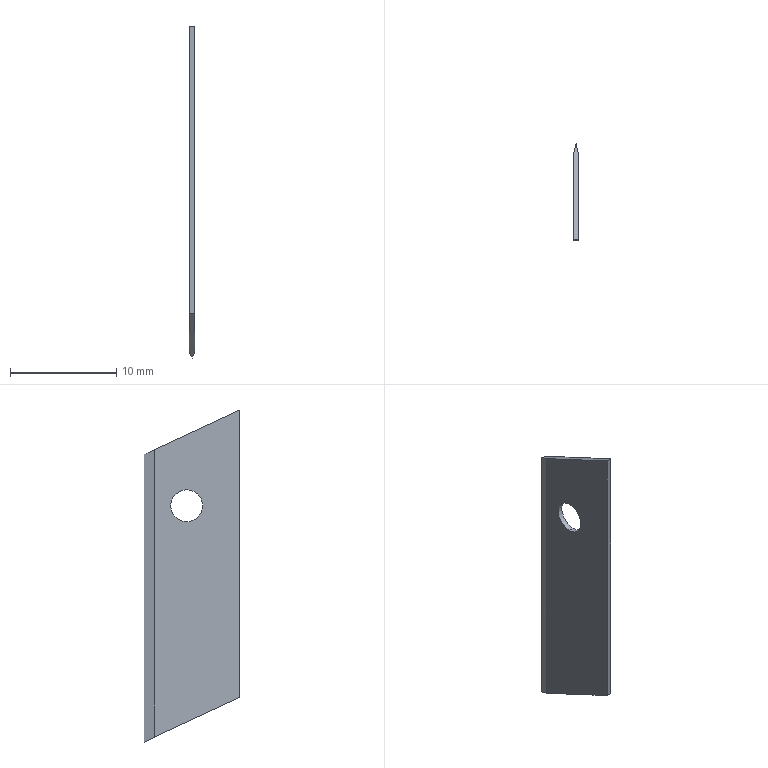Part | STEP file | Insert blade | 1 solid | 9 faces | box 0.5 x 9 x 31.197 mm | volume 111.216 mm3 | plane 7 | cylinder 2 | commonest cylinder face diameters 3 x2
STEP:
#1=CARTESIAN_POINT('',(0.,0.,0.));
#2=DIRECTION('',(0.,0.,1.));
#3=DIRECTION('',(1.,0.,0.));
#4=AXIS2_PLACEMENT_3D('',#1,#2,#3);
#5=CARTESIAN_POINT('',(-0.25,5.,-10.5));
#6=VERTEX_POINT('',#5);
#7=CARTESIAN_POINT('',(0.25,5.,-10.5));
#8=VERTEX_POINT('',#7);
#9=CARTESIAN_POINT('',(-0.25,5.,-10.5));
#10=DIRECTION('',(1.,0.,0.));
#11=VECTOR('',#10,1.);
#12=LINE('',#9,#11);
#13=CARTESIAN_POINT('',(-0.25,5.,-9.));
#14=DIRECTION('',(1.,0.,0.));
#15=DIRECTION('',(0.,0.,-1.));
#16=AXIS2_PLACEMENT_3D('',#13,#14,#15);
#17=CYLINDRICAL_SURFACE('',#16,1.5);
#18=CARTESIAN_POINT('',(6.283,0.));
#19=DIRECTION('',(0.,1.));
#20=VECTOR('',#19,1.);
#21=LINE('',#18,#20);
#22=(GEOMETRIC_REPRESENTATION_CONTEXT(2)PARAMETRIC_REPRESENTATION_CONTEXT()REPRESENTATION_CONTEXT('',''));
#23=DEFINITIONAL_REPRESENTATION('',(#21),#22);
#24=PCURVE('',#17,#23);
#25=CARTESIAN_POINT('',(-0.25,5.,-9.));
#26=DIRECTION('',(1.,0.,0.));
#27=DIRECTION('',(0.,0.,-1.));
#28=AXIS2_PLACEMENT_3D('',#25,#26,#27);
#29=CYLINDRICAL_SURFACE('',#28,1.5);
#30=CARTESIAN_POINT('',(0.,0.));
#31=DIRECTION('',(0.,1.));
#32=VECTOR('',#31,1.);
#33=LINE('',#30,#32);
#34=(GEOMETRIC_REPRESENTATION_CONTEXT(2)PARAMETRIC_REPRESENTATION_CONTEXT()REPRESENTATION_CONTEXT('',''));
#35=DEFINITIONAL_REPRESENTATION('',(#33),#34);
#36=PCURVE('',#29,#35);
#37=SURFACE_CURVE('',#12,(#24,#36),.PCURVE_S1.);
#38=EDGE_CURVE('',#6,#8,#37,.T.);
#39=ORIENTED_EDGE('',*,*,#38,.T.);
#40=CARTESIAN_POINT('',(0.25,5.,-7.5));
#41=VERTEX_POINT('',#40);
#42=CARTESIAN_POINT('',(0.25,5.,-9.));
#43=DIRECTION('',(1.,0.,0.));
#44=DIRECTION('',(0.,0.,-1.));
#45=AXIS2_PLACEMENT_3D('',#42,#43,#44);
#46=CIRCLE('',#45,1.5);
#47=CARTESIAN_POINT('',(0.,0.5));
#48=DIRECTION('',(1.,0.));
#49=VECTOR('',#48,1.);
#50=LINE('',#47,#49);
#51=(GEOMETRIC_REPRESENTATION_CONTEXT(2)PARAMETRIC_REPRESENTATION_CONTEXT()REPRESENTATION_CONTEXT('',''));
#52=DEFINITIONAL_REPRESENTATION('',(#50),#51);
#53=PCURVE('',#17,#52);
#54=CARTESIAN_POINT('',(0.25,0.,-30.915));
#55=DIRECTION('',(-1.,0.,0.));
#56=DIRECTION('',(0.,0.,1.));
#57=AXIS2_PLACEMENT_3D('',#54,#55,#56);
#58=PLANE('',#57);
#59=CARTESIAN_POINT('',(20.415,5.));
#60=CARTESIAN_POINT('',(20.415,7.598));
#61=CARTESIAN_POINT('',(22.665,6.299));
#62=CARTESIAN_POINT('',(24.915,5.));
#63=CARTESIAN_POINT('',(22.665,3.701));
#64=CARTESIAN_POINT('',(20.415,2.402));
#65=CARTESIAN_POINT('',(20.415,5.));
#66=(BOUNDED_CURVE()B_SPLINE_CURVE(2,(#59,#60,#61,#62,#63,#64,#65),.UNSPECIFIED.,.T.,.F.)B_SPLINE_CURVE_WITH_KNOTS((1,2,2,2,2,1),(-2.094,0.,2.094,4.189,6.283,8.378),.UNSPECIFIED.)CURVE()GEOMETRIC_REPRESENTATION_ITEM()RATIONAL_B_SPLINE_CURVE((1.,0.5,1.,0.5,1.,0.5,1.))REPRESENTATION_ITEM(''));
#67=(GEOMETRIC_REPRESENTATION_CONTEXT(2)PARAMETRIC_REPRESENTATION_CONTEXT()REPRESENTATION_CONTEXT('',''));
#68=DEFINITIONAL_REPRESENTATION('',(#66),#67);
#69=PCURVE('',#58,#68);
#70=SURFACE_CURVE('',#46,(#53,#69),.PCURVE_S1.);
#71=EDGE_CURVE('',#41,#8,#70,.T.);
#72=ORIENTED_EDGE('',*,*,#71,.F.);
#73=CARTESIAN_POINT('',(-0.25,5.,-7.5));
#74=VERTEX_POINT('',#73);
#75=CARTESIAN_POINT('',(-0.25,5.,-7.5));
#76=DIRECTION('',(1.,0.,0.));
#77=VECTOR('',#76,1.);
#78=LINE('',#75,#77);
#79=CARTESIAN_POINT('',(3.142,0.));
#80=DIRECTION('',(0.,1.));
#81=VECTOR('',#80,1.);
#82=LINE('',#79,#81);
#83=(GEOMETRIC_REPRESENTATION_CONTEXT(2)PARAMETRIC_REPRESENTATION_CONTEXT()REPRESENTATION_CONTEXT('',''));
#84=DEFINITIONAL_REPRESENTATION('',(#82),#83);
#85=PCURVE('',#17,#84);
#86=CARTESIAN_POINT('',(3.142,0.));
#87=DIRECTION('',(0.,1.));
#88=VECTOR('',#87,1.);
#89=LINE('',#86,#88);
#90=(GEOMETRIC_REPRESENTATION_CONTEXT(2)PARAMETRIC_REPRESENTATION_CONTEXT()REPRESENTATION_CONTEXT('',''));
#91=DEFINITIONAL_REPRESENTATION('',(#89),#90);
#92=PCURVE('',#29,#91);
#93=SURFACE_CURVE('',#78,(#85,#92),.PCURVE_S1.);
#94=EDGE_CURVE('',#74,#41,#93,.T.);
#95=ORIENTED_EDGE('',*,*,#94,.F.);
#96=CARTESIAN_POINT('',(-0.25,5.,-9.));
#97=DIRECTION('',(-1.,0.,0.));
#98=DIRECTION('',(0.,0.,-1.));
#99=AXIS2_PLACEMENT_3D('',#96,#97,#98);
#100=CIRCLE('',#99,1.5);
#101=CARTESIAN_POINT('',(6.283,0.));
#102=DIRECTION('',(-1.,0.));
#103=VECTOR('',#102,1.);
#104=LINE('',#101,#103);
#105=(GEOMETRIC_REPRESENTATION_CONTEXT(2)PARAMETRIC_REPRESENTATION_CONTEXT()REPRESENTATION_CONTEXT('',''));
#106=DEFINITIONAL_REPRESENTATION('',(#104),#105);
#107=PCURVE('',#17,#106);
#108=CARTESIAN_POINT('',(-0.25,0.,-30.915));
#109=DIRECTION('',(-1.,0.,0.));
#110=DIRECTION('',(0.,0.,1.));
#111=AXIS2_PLACEMENT_3D('',#108,#109,#110);
#112=PLANE('',#111);
#113=CARTESIAN_POINT('',(21.915,5.));
#114=DIRECTION('',(-1.,0.));
#115=AXIS2_PLACEMENT_2D('',#113,#114);
#116=CIRCLE('',#115,1.5);
#117=(GEOMETRIC_REPRESENTATION_CONTEXT(2)PARAMETRIC_REPRESENTATION_CONTEXT()REPRESENTATION_CONTEXT('',''));
#118=DEFINITIONAL_REPRESENTATION('',(#116),#117);
#119=PCURVE('',#112,#118);
#120=SURFACE_CURVE('',#100,(#107,#119),.PCURVE_S1.);
#121=EDGE_CURVE('',#6,#74,#120,.T.);
#122=ORIENTED_EDGE('',*,*,#121,.F.);
#123=EDGE_LOOP('',(#39,#72,#95,#122));
#124=FACE_BOUND('',#123,.F.);
#125=ADVANCED_FACE('',(#124),#17,.F.);
#126=CARTESIAN_POINT('',(0.25,5.,-9.));
#127=DIRECTION('',(1.,0.,0.));
#128=DIRECTION('',(0.,0.,-1.));
#129=AXIS2_PLACEMENT_3D('',#126,#127,#128);
#130=CIRCLE('',#129,1.5);
#131=CARTESIAN_POINT('',(0.,0.5));
#132=DIRECTION('',(1.,0.));
#133=VECTOR('',#132,1.);
#134=LINE('',#131,#133);
#135=(GEOMETRIC_REPRESENTATION_CONTEXT(2)PARAMETRIC_REPRESENTATION_CONTEXT()REPRESENTATION_CONTEXT('',''));
#136=DEFINITIONAL_REPRESENTATION('',(#134),#135);
#137=PCURVE('',#29,#136);
#138=CARTESIAN_POINT('',(20.415,5.));
#139=CARTESIAN_POINT('',(20.415,7.598));
#140=CARTESIAN_POINT('',(22.665,6.299));
#141=CARTESIAN_POINT('',(24.915,5.));
#142=CARTESIAN_POINT('',(22.665,3.701));
#143=CARTESIAN_POINT('',(20.415,2.402));
#144=CARTESIAN_POINT('',(20.415,5.));
#145=(BOUNDED_CURVE()B_SPLINE_CURVE(2,(#138,#139,#140,#141,#142,#143,#144),.UNSPECIFIED.,.T.,.F.)B_SPLINE_CURVE_WITH_KNOTS((1,2,2,2,2,1),(-2.094,0.,2.094,4.189,6.283,8.378),.UNSPECIFIED.)CURVE()GEOMETRIC_REPRESENTATION_ITEM()RATIONAL_B_SPLINE_CURVE((1.,0.5,1.,0.5,1.,0.5,1.))REPRESENTATION_ITEM(''));
#146=(GEOMETRIC_REPRESENTATION_CONTEXT(2)PARAMETRIC_REPRESENTATION_CONTEXT()REPRESENTATION_CONTEXT('',''));
#147=DEFINITIONAL_REPRESENTATION('',(#145),#146);
#148=PCURVE('',#58,#147);
#149=SURFACE_CURVE('',#130,(#137,#148),.PCURVE_S1.);
#150=EDGE_CURVE('',#8,#41,#149,.T.);
#151=ORIENTED_EDGE('',*,*,#150,.F.);
#152=ORIENTED_EDGE('',*,*,#38,.F.);
#153=CARTESIAN_POINT('',(-0.25,5.,-9.));
#154=DIRECTION('',(-1.,0.,0.));
#155=DIRECTION('',(0.,0.,-1.));
#156=AXIS2_PLACEMENT_3D('',#153,#154,#155);
#157=CIRCLE('',#156,1.5);
#158=CARTESIAN_POINT('',(6.283,0.));
#159=DIRECTION('',(-1.,0.));
#160=VECTOR('',#159,1.);
#161=LINE('',#158,#160);
#162=(GEOMETRIC_REPRESENTATION_CONTEXT(2)PARAMETRIC_REPRESENTATION_CONTEXT()REPRESENTATION_CONTEXT('',''));
#163=DEFINITIONAL_REPRESENTATION('',(#161),#162);
#164=PCURVE('',#29,#163);
#165=CARTESIAN_POINT('',(21.915,5.));
#166=DIRECTION('',(-1.,0.));
#167=AXIS2_PLACEMENT_2D('',#165,#166);
#168=CIRCLE('',#167,1.5);
#169=(GEOMETRIC_REPRESENTATION_CONTEXT(2)PARAMETRIC_REPRESENTATION_CONTEXT()REPRESENTATION_CONTEXT('',''));
#170=DEFINITIONAL_REPRESENTATION('',(#168),#169);
#171=PCURVE('',#112,#170);
#172=SURFACE_CURVE('',#157,(#164,#171),.PCURVE_S1.);
#173=EDGE_CURVE('',#74,#6,#172,.T.);
#174=ORIENTED_EDGE('',*,*,#173,.F.);
#175=ORIENTED_EDGE('',*,*,#94,.T.);
#176=EDGE_LOOP('',(#151,#152,#174,#175));
#177=FACE_BOUND('',#176,.F.);
#178=ADVANCED_FACE('',(#177),#29,.F.);
#179=ORIENTED_EDGE('',*,*,#150,.F.);
#180=ORIENTED_EDGE('',*,*,#71,.F.);
#181=EDGE_LOOP('',(#179,#180));
#182=FACE_BOUND('',#181,.T.);
#183=CARTESIAN_POINT('',(0.25,8.,-3.73));
#184=VERTEX_POINT('',#183);
#185=CARTESIAN_POINT('',(0.25,8.,-30.73));
#186=VERTEX_POINT('',#185);
#187=CARTESIAN_POINT('',(0.25,8.,-15.365));
#188=DIRECTION('',(0.,0.,-1.));
#189=VECTOR('',#188,1.);
#190=LINE('',#187,#189);
#191=CARTESIAN_POINT('',(15.55,8.));
#192=DIRECTION('',(-1.,0.));
#193=VECTOR('',#192,1.);
#194=LINE('',#191,#193);
#195=(GEOMETRIC_REPRESENTATION_CONTEXT(2)PARAMETRIC_REPRESENTATION_CONTEXT()REPRESENTATION_CONTEXT('',''));
#196=DEFINITIONAL_REPRESENTATION('',(#194),#195);
#197=PCURVE('',#58,#196);
#198=CARTESIAN_POINT('',(0.,9.,-31.362));
#199=DIRECTION('',(-0.9701,-0.2425,0.));
#200=DIRECTION('',(0.2425,-0.9701,0.));
#201=AXIS2_PLACEMENT_3D('',#198,#199,#200);
#202=PLANE('',#201);
#203=CARTESIAN_POINT('',(1.031,15.996));
#204=DIRECTION('',(0.,-1.));
#205=VECTOR('',#204,1.);
#206=LINE('',#203,#205);
#207=(GEOMETRIC_REPRESENTATION_CONTEXT(2)PARAMETRIC_REPRESENTATION_CONTEXT()REPRESENTATION_CONTEXT('',''));
#208=DEFINITIONAL_REPRESENTATION('',(#206),#207);
#209=PCURVE('',#202,#208);
#210=SURFACE_CURVE('',#190,(#197,#209),.PCURVE_S1.);
#211=EDGE_CURVE('',#184,#186,#210,.T.);
#212=ORIENTED_EDGE('',*,*,#211,.F.);
#213=CARTESIAN_POINT('',(0.25,0.,0.));
#214=VERTEX_POINT('',#213);
#215=CARTESIAN_POINT('',(0.25,0.,0.));
#216=DIRECTION('',(0.,0.9063,-0.4226));
#217=VECTOR('',#216,1.);
#218=LINE('',#215,#217);
#219=CARTESIAN_POINT('',(30.915,0.));
#220=DIRECTION('',(-0.4226,0.9063));
#221=VECTOR('',#220,1.);
#222=LINE('',#219,#221);
#223=(GEOMETRIC_REPRESENTATION_CONTEXT(2)PARAMETRIC_REPRESENTATION_CONTEXT()REPRESENTATION_CONTEXT('',''));
#224=DEFINITIONAL_REPRESENTATION('',(#222),#223);
#225=PCURVE('',#58,#224);
#226=CARTESIAN_POINT('',(-0.25,0.,0.));
#227=DIRECTION('',(0.,-0.4226,-0.9063));
#228=DIRECTION('',(0.,0.9063,-0.4226));
#229=AXIS2_PLACEMENT_3D('',#226,#227,#228);
#230=PLANE('',#229);
#231=CARTESIAN_POINT('',(0.,0.5));
#232=DIRECTION('',(1.,0.));
#233=VECTOR('',#232,1.);
#234=LINE('',#231,#233);
#235=(GEOMETRIC_REPRESENTATION_CONTEXT(2)PARAMETRIC_REPRESENTATION_CONTEXT()REPRESENTATION_CONTEXT('',''));
#236=DEFINITIONAL_REPRESENTATION('',(#234),#235);
#237=PCURVE('',#230,#236);
#238=SURFACE_CURVE('',#218,(#225,#237),.PCURVE_S1.);
#239=EDGE_CURVE('',#214,#184,#238,.T.);
#240=ORIENTED_EDGE('',*,*,#239,.F.);
#241=CARTESIAN_POINT('',(0.25,0.,-27.));
#242=VERTEX_POINT('',#241);
#243=CARTESIAN_POINT('',(0.25,0.,-15.365));
#244=DIRECTION('',(0.,0.,1.));
#245=VECTOR('',#244,1.);
#246=LINE('',#243,#245);
#247=CARTESIAN_POINT('',(15.55,0.));
#248=DIRECTION('',(1.,0.));
#249=VECTOR('',#248,1.);
#250=LINE('',#247,#249);
#251=(GEOMETRIC_REPRESENTATION_CONTEXT(2)PARAMETRIC_REPRESENTATION_CONTEXT()REPRESENTATION_CONTEXT('',''));
#252=DEFINITIONAL_REPRESENTATION('',(#250),#251);
#253=PCURVE('',#58,#252);
#254=CARTESIAN_POINT('',(-0.25,0.,-27.));
#255=DIRECTION('',(0.,1.,0.));
#256=DIRECTION('',(0.,0.,1.));
#257=AXIS2_PLACEMENT_3D('',#254,#255,#256);
#258=PLANE('',#257);
#259=CARTESIAN_POINT('',(11.635,0.5));
#260=DIRECTION('',(1.,0.));
#261=VECTOR('',#260,1.);
#262=LINE('',#259,#261);
#263=(GEOMETRIC_REPRESENTATION_CONTEXT(2)PARAMETRIC_REPRESENTATION_CONTEXT()REPRESENTATION_CONTEXT('',''));
#264=DEFINITIONAL_REPRESENTATION('',(#262),#263);
#265=PCURVE('',#258,#264);
#266=SURFACE_CURVE('',#246,(#253,#265),.PCURVE_S1.);
#267=EDGE_CURVE('',#242,#214,#266,.T.);
#268=ORIENTED_EDGE('',*,*,#267,.F.);
#269=CARTESIAN_POINT('',(0.25,9.,-31.197));
#270=DIRECTION('',(0.,-0.9063,0.4226));
#271=VECTOR('',#270,1.);
#272=LINE('',#269,#271);
#273=CARTESIAN_POINT('',(-0.2819,9.));
#274=DIRECTION('',(0.4226,-0.9063));
#275=VECTOR('',#274,1.);
#276=LINE('',#273,#275);
#277=(GEOMETRIC_REPRESENTATION_CONTEXT(2)PARAMETRIC_REPRESENTATION_CONTEXT()REPRESENTATION_CONTEXT('',''));
#278=DEFINITIONAL_REPRESENTATION('',(#276),#277);
#279=PCURVE('',#58,#278);
#280=CARTESIAN_POINT('',(-0.25,9.,-31.197));
#281=DIRECTION('',(0.,0.4226,0.9063));
#282=DIRECTION('',(0.,-0.9063,0.4226));
#283=AXIS2_PLACEMENT_3D('',#280,#281,#282);
#284=PLANE('',#283);
#285=CARTESIAN_POINT('',(0.,0.5));
#286=DIRECTION('',(1.,0.));
#287=VECTOR('',#286,1.);
#288=LINE('',#285,#287);
#289=(GEOMETRIC_REPRESENTATION_CONTEXT(2)PARAMETRIC_REPRESENTATION_CONTEXT()REPRESENTATION_CONTEXT('',''));
#290=DEFINITIONAL_REPRESENTATION('',(#288),#289);
#291=PCURVE('',#284,#290);
#292=SURFACE_CURVE('',#272,(#279,#291),.PCURVE_S1.);
#293=EDGE_CURVE('',#186,#242,#292,.T.);
#294=ORIENTED_EDGE('',*,*,#293,.F.);
#295=EDGE_LOOP('',(#212,#240,#268,#294));
#296=FACE_BOUND('',#295,.T.);
#297=ADVANCED_FACE('',(#182,#296),#58,.F.);
#298=ORIENTED_EDGE('',*,*,#121,.F.);
#299=ORIENTED_EDGE('',*,*,#173,.F.);
#300=EDGE_LOOP('',(#298,#299));
#301=FACE_BOUND('',#300,.T.);
#302=CARTESIAN_POINT('',(-0.25,8.,-30.73));
#303=VERTEX_POINT('',#302);
#304=CARTESIAN_POINT('',(-0.25,0.,-27.));
#305=VERTEX_POINT('',#304);
#306=CARTESIAN_POINT('',(-0.25,8.,-30.73));
#307=DIRECTION('',(0.,-0.9063,0.4226));
#308=VECTOR('',#307,1.);
#309=LINE('',#306,#308);
#310=CARTESIAN_POINT('',(0.1844,8.));
#311=DIRECTION('',(0.4226,-0.9063));
#312=VECTOR('',#311,1.);
#313=LINE('',#310,#312);
#314=(GEOMETRIC_REPRESENTATION_CONTEXT(2)PARAMETRIC_REPRESENTATION_CONTEXT()REPRESENTATION_CONTEXT('',''));
#315=DEFINITIONAL_REPRESENTATION('',(#313),#314);
#316=PCURVE('',#112,#315);
#317=CARTESIAN_POINT('',(1.103,0.));
#318=DIRECTION('',(1.,0.));
#319=VECTOR('',#318,1.);
#320=LINE('',#317,#319);
#321=(GEOMETRIC_REPRESENTATION_CONTEXT(2)PARAMETRIC_REPRESENTATION_CONTEXT()REPRESENTATION_CONTEXT('',''));
#322=DEFINITIONAL_REPRESENTATION('',(#320),#321);
#323=PCURVE('',#284,#322);
#324=SURFACE_CURVE('',#309,(#316,#323),.PCURVE_S1.);
#325=EDGE_CURVE('',#303,#305,#324,.T.);
#326=ORIENTED_EDGE('',*,*,#325,.T.);
#327=CARTESIAN_POINT('',(-0.25,0.,-0.000000004));
#328=VERTEX_POINT('',#327);
#329=CARTESIAN_POINT('',(-0.25,0.,-15.365));
#330=DIRECTION('',(0.,0.,1.));
#331=VECTOR('',#330,1.);
#332=LINE('',#329,#331);
#333=CARTESIAN_POINT('',(15.55,0.));
#334=DIRECTION('',(1.,0.));
#335=VECTOR('',#334,1.);
#336=LINE('',#333,#335);
#337=(GEOMETRIC_REPRESENTATION_CONTEXT(2)PARAMETRIC_REPRESENTATION_CONTEXT()REPRESENTATION_CONTEXT('',''));
#338=DEFINITIONAL_REPRESENTATION('',(#336),#337);
#339=PCURVE('',#112,#338);
#340=CARTESIAN_POINT('',(11.635,0.));
#341=DIRECTION('',(1.,0.));
#342=VECTOR('',#341,1.);
#343=LINE('',#340,#342);
#344=(GEOMETRIC_REPRESENTATION_CONTEXT(2)PARAMETRIC_REPRESENTATION_CONTEXT()REPRESENTATION_CONTEXT('',''));
#345=DEFINITIONAL_REPRESENTATION('',(#343),#344);
#346=PCURVE('',#258,#345);
#347=SURFACE_CURVE('',#332,(#339,#346),.PCURVE_S1.);
#348=EDGE_CURVE('',#305,#328,#347,.T.);
#349=ORIENTED_EDGE('',*,*,#348,.T.);
#350=CARTESIAN_POINT('',(-0.25,8.,-3.73));
#351=VERTEX_POINT('',#350);
#352=CARTESIAN_POINT('',(-0.25,0.,-0.000000007));
#353=DIRECTION('',(0.,0.9063,-0.4226));
#354=VECTOR('',#353,1.);
#355=LINE('',#352,#354);
#356=CARTESIAN_POINT('',(30.915,0.));
#357=DIRECTION('',(-0.4226,0.9063));
#358=VECTOR('',#357,1.);
#359=LINE('',#356,#358);
#360=(GEOMETRIC_REPRESENTATION_CONTEXT(2)PARAMETRIC_REPRESENTATION_CONTEXT()REPRESENTATION_CONTEXT('',''));
#361=DEFINITIONAL_REPRESENTATION('',(#359),#360);
#362=PCURVE('',#112,#361);
#363=CARTESIAN_POINT('',(0.000000003,0.));
#364=DIRECTION('',(1.,0.));
#365=VECTOR('',#364,1.);
#366=LINE('',#363,#365);
#367=(GEOMETRIC_REPRESENTATION_CONTEXT(2)PARAMETRIC_REPRESENTATION_CONTEXT()REPRESENTATION_CONTEXT('',''));
#368=DEFINITIONAL_REPRESENTATION('',(#366),#367);
#369=PCURVE('',#230,#368);
#370=SURFACE_CURVE('',#355,(#362,#369),.PCURVE_S1.);
#371=EDGE_CURVE('',#328,#351,#370,.T.);
#372=ORIENTED_EDGE('',*,*,#371,.T.);
#373=CARTESIAN_POINT('',(-0.25,8.,-15.365));
#374=DIRECTION('',(0.,0.,-1.));
#375=VECTOR('',#374,1.);
#376=LINE('',#373,#375);
#377=CARTESIAN_POINT('',(15.55,8.));
#378=DIRECTION('',(-1.,0.));
#379=VECTOR('',#378,1.);
#380=LINE('',#377,#379);
#381=(GEOMETRIC_REPRESENTATION_CONTEXT(2)PARAMETRIC_REPRESENTATION_CONTEXT()REPRESENTATION_CONTEXT('',''));
#382=DEFINITIONAL_REPRESENTATION('',(#380),#381);
#383=PCURVE('',#112,#382);
#384=CARTESIAN_POINT('',(0.,9.,-31.362));
#385=DIRECTION('',(-0.9701,0.2425,0.));
#386=DIRECTION('',(-0.2425,-0.9701,0.));
#387=AXIS2_PLACEMENT_3D('',#384,#385,#386);
#388=PLANE('',#387);
#389=CARTESIAN_POINT('',(1.031,15.996));
#390=DIRECTION('',(0.,-1.));
#391=VECTOR('',#390,1.);
#392=LINE('',#389,#391);
#393=(GEOMETRIC_REPRESENTATION_CONTEXT(2)PARAMETRIC_REPRESENTATION_CONTEXT()REPRESENTATION_CONTEXT('',''));
#394=DEFINITIONAL_REPRESENTATION('',(#392),#393);
#395=PCURVE('',#388,#394);
#396=SURFACE_CURVE('',#376,(#383,#395),.PCURVE_S1.);
#397=EDGE_CURVE('',#351,#303,#396,.T.);
#398=ORIENTED_EDGE('',*,*,#397,.T.);
#399=EDGE_LOOP('',(#326,#349,#372,#398));
#400=FACE_BOUND('',#399,.T.);
#401=ADVANCED_FACE('',(#301,#400),#112,.T.);
#402=CARTESIAN_POINT('',(0.,9.,-31.197));
#403=VERTEX_POINT('',#402);
#404=CARTESIAN_POINT('',(0.,9.,-31.197));
#405=DIRECTION('',(-0.221,-0.8839,0.4122));
#406=VECTOR('',#405,1.);
#407=LINE('',#404,#406);
#408=CARTESIAN_POINT('',(0.,0.25));
#409=DIRECTION('',(0.9753,-0.221));
#410=VECTOR('',#409,1.);
#411=LINE('',#408,#410);
#412=(GEOMETRIC_REPRESENTATION_CONTEXT(2)PARAMETRIC_REPRESENTATION_CONTEXT()REPRESENTATION_CONTEXT('',''));
#413=DEFINITIONAL_REPRESENTATION('',(#411),#412);
#414=PCURVE('',#284,#413);
#415=CARTESIAN_POINT('',(0.,0.1648));
#416=DIRECTION('',(0.9111,0.4122));
#417=VECTOR('',#416,1.);
#418=LINE('',#415,#417);
#419=(GEOMETRIC_REPRESENTATION_CONTEXT(2)PARAMETRIC_REPRESENTATION_CONTEXT()REPRESENTATION_CONTEXT('',''));
#420=DEFINITIONAL_REPRESENTATION('',(#418),#419);
#421=PCURVE('',#388,#420);
#422=SURFACE_CURVE('',#407,(#414,#421),.PCURVE_S1.);
#423=EDGE_CURVE('',#403,#303,#422,.T.);
#424=ORIENTED_EDGE('',*,*,#423,.F.);
#425=CARTESIAN_POINT('',(0.25,8.,-30.73));
#426=DIRECTION('',(-0.221,0.8839,-0.4122));
#427=VECTOR('',#426,1.);
#428=LINE('',#425,#427);
#429=CARTESIAN_POINT('',(1.103,0.5));
#430=DIRECTION('',(-0.9753,-0.221));
#431=VECTOR('',#430,1.);
#432=LINE('',#429,#431);
#433=(GEOMETRIC_REPRESENTATION_CONTEXT(2)PARAMETRIC_REPRESENTATION_CONTEXT()REPRESENTATION_CONTEXT('',''));
#434=DEFINITIONAL_REPRESENTATION('',(#432),#433);
#435=PCURVE('',#284,#434);
#436=CARTESIAN_POINT('',(1.031,0.6311));
#437=DIRECTION('',(-0.9111,-0.4122));
#438=VECTOR('',#437,1.);
#439=LINE('',#436,#438);
#440=(GEOMETRIC_REPRESENTATION_CONTEXT(2)PARAMETRIC_REPRESENTATION_CONTEXT()REPRESENTATION_CONTEXT('',''));
#441=DEFINITIONAL_REPRESENTATION('',(#439),#440);
#442=PCURVE('',#202,#441);
#443=SURFACE_CURVE('',#428,(#435,#442),.PCURVE_S1.);
#444=EDGE_CURVE('',#186,#403,#443,.T.);
#445=ORIENTED_EDGE('',*,*,#444,.F.);
#446=ORIENTED_EDGE('',*,*,#293,.T.);
#447=CARTESIAN_POINT('',(0.,0.,-27.));
#448=DIRECTION('',(1.,0.,0.));
#449=VECTOR('',#448,1.);
#450=LINE('',#447,#449);
#451=CARTESIAN_POINT('',(9.93,0.25));
#452=DIRECTION('',(0.,1.));
#453=VECTOR('',#452,1.);
#454=LINE('',#451,#453);
#455=(GEOMETRIC_REPRESENTATION_CONTEXT(2)PARAMETRIC_REPRESENTATION_CONTEXT()REPRESENTATION_CONTEXT('',''));
#456=DEFINITIONAL_REPRESENTATION('',(#454),#455);
#457=PCURVE('',#284,#456);
#458=CARTESIAN_POINT('',(0.,0.25));
#459=DIRECTION('',(0.,1.));
#460=VECTOR('',#459,1.);
#461=LINE('',#458,#460);
#462=(GEOMETRIC_REPRESENTATION_CONTEXT(2)PARAMETRIC_REPRESENTATION_CONTEXT()REPRESENTATION_CONTEXT('',''));
#463=DEFINITIONAL_REPRESENTATION('',(#461),#462);
#464=PCURVE('',#258,#463);
#465=SURFACE_CURVE('',#450,(#457,#464),.PCURVE_S1.);
#466=EDGE_CURVE('',#305,#242,#465,.T.);
#467=ORIENTED_EDGE('',*,*,#466,.F.);
#468=ORIENTED_EDGE('',*,*,#325,.F.);
#469=EDGE_LOOP('',(#424,#445,#446,#467,#468));
#470=FACE_BOUND('',#469,.T.);
#471=ADVANCED_FACE('',(#470),#284,.F.);
#472=CARTESIAN_POINT('',(0.,9.,-4.197));
#473=VERTEX_POINT('',#472);
#474=CARTESIAN_POINT('',(0.,9.,-17.464));
#475=DIRECTION('',(0.,0.,-1.));
#476=VECTOR('',#475,1.);
#477=LINE('',#474,#476);
#478=CARTESIAN_POINT('',(0.,13.898));
#479=DIRECTION('',(0.,-1.));
#480=VECTOR('',#479,1.);
#481=LINE('',#478,#480);
#482=(GEOMETRIC_REPRESENTATION_CONTEXT(2)PARAMETRIC_REPRESENTATION_CONTEXT()REPRESENTATION_CONTEXT('',''));
#483=DEFINITIONAL_REPRESENTATION('',(#481),#482);
#484=PCURVE('',#202,#483);
#485=CARTESIAN_POINT('',(0.,13.898));
#486=DIRECTION('',(0.,-1.));
#487=VECTOR('',#486,1.);
#488=LINE('',#485,#487);
#489=(GEOMETRIC_REPRESENTATION_CONTEXT(2)PARAMETRIC_REPRESENTATION_CONTEXT()REPRESENTATION_CONTEXT('',''));
#490=DEFINITIONAL_REPRESENTATION('',(#488),#489);
#491=PCURVE('',#388,#490);
#492=SURFACE_CURVE('',#477,(#484,#491),.PCURVE_S1.);
#493=EDGE_CURVE('',#473,#403,#492,.T.);
#494=ORIENTED_EDGE('',*,*,#493,.F.);
#495=CARTESIAN_POINT('',(0.25,8.,-3.73));
#496=DIRECTION('',(-0.221,0.8839,-0.4122));
#497=VECTOR('',#496,1.);
#498=LINE('',#495,#497);
#499=CARTESIAN_POINT('',(1.031,27.631));
#500=DIRECTION('',(-0.9111,-0.4122));
#501=VECTOR('',#500,1.);
#502=LINE('',#499,#501);
#503=(GEOMETRIC_REPRESENTATION_CONTEXT(2)PARAMETRIC_REPRESENTATION_CONTEXT()REPRESENTATION_CONTEXT('',''));
#504=DEFINITIONAL_REPRESENTATION('',(#502),#503);
#505=PCURVE('',#202,#504);
#506=CARTESIAN_POINT('',(8.827,0.5));
#507=DIRECTION('',(0.9753,-0.221));
#508=VECTOR('',#507,1.);
#509=LINE('',#506,#508);
#510=(GEOMETRIC_REPRESENTATION_CONTEXT(2)PARAMETRIC_REPRESENTATION_CONTEXT()REPRESENTATION_CONTEXT('',''));
#511=DEFINITIONAL_REPRESENTATION('',(#509),#510);
#512=PCURVE('',#230,#511);
#513=SURFACE_CURVE('',#498,(#505,#512),.PCURVE_S1.);
#514=EDGE_CURVE('',#184,#473,#513,.T.);
#515=ORIENTED_EDGE('',*,*,#514,.F.);
#516=ORIENTED_EDGE('',*,*,#211,.T.);
#517=ORIENTED_EDGE('',*,*,#444,.T.);
#518=EDGE_LOOP('',(#494,#515,#516,#517));
#519=FACE_BOUND('',#518,.T.);
#520=ADVANCED_FACE('',(#519),#202,.F.);
#521=CARTESIAN_POINT('',(-0.25,8.,-3.73));
#522=DIRECTION('',(0.221,0.8839,-0.4122));
#523=VECTOR('',#522,1.);
#524=LINE('',#521,#523);
#525=CARTESIAN_POINT('',(8.827,0.));
#526=DIRECTION('',(0.9753,0.221));
#527=VECTOR('',#526,1.);
#528=LINE('',#525,#527);
#529=(GEOMETRIC_REPRESENTATION_CONTEXT(2)PARAMETRIC_REPRESENTATION_CONTEXT()REPRESENTATION_CONTEXT('',''));
#530=DEFINITIONAL_REPRESENTATION('',(#528),#529);
#531=PCURVE('',#230,#530);
#532=CARTESIAN_POINT('',(1.031,27.631));
#533=DIRECTION('',(-0.9111,-0.4122));
#534=VECTOR('',#533,1.);
#535=LINE('',#532,#534);
#536=(GEOMETRIC_REPRESENTATION_CONTEXT(2)PARAMETRIC_REPRESENTATION_CONTEXT()REPRESENTATION_CONTEXT('',''));
#537=DEFINITIONAL_REPRESENTATION('',(#535),#536);
#538=PCURVE('',#388,#537);
#539=SURFACE_CURVE('',#524,(#531,#538),.PCURVE_S1.);
#540=EDGE_CURVE('',#351,#473,#539,.T.);
#541=ORIENTED_EDGE('',*,*,#540,.F.);
#542=ORIENTED_EDGE('',*,*,#371,.F.);
#543=CARTESIAN_POINT('',(0.,0.,0.));
#544=DIRECTION('',(-1.,0.,0.));
#545=VECTOR('',#544,1.);
#546=LINE('',#543,#545);
#547=CARTESIAN_POINT('',(0.,0.25));
#548=DIRECTION('',(0.,-1.));
#549=VECTOR('',#548,1.);
#550=LINE('',#547,#549);
#551=(GEOMETRIC_REPRESENTATION_CONTEXT(2)PARAMETRIC_REPRESENTATION_CONTEXT()REPRESENTATION_CONTEXT('',''));
#552=DEFINITIONAL_REPRESENTATION('',(#550),#551);
#553=PCURVE('',#230,#552);
#554=CARTESIAN_POINT('',(27.,0.25));
#555=DIRECTION('',(0.,-1.));
#556=VECTOR('',#555,1.);
#557=LINE('',#554,#556);
#558=(GEOMETRIC_REPRESENTATION_CONTEXT(2)PARAMETRIC_REPRESENTATION_CONTEXT()REPRESENTATION_CONTEXT('',''));
#559=DEFINITIONAL_REPRESENTATION('',(#557),#558);
#560=PCURVE('',#258,#559);
#561=SURFACE_CURVE('',#546,(#553,#560),.PCURVE_S1.);
#562=EDGE_CURVE('',#214,#328,#561,.T.);
#563=ORIENTED_EDGE('',*,*,#562,.F.);
#564=ORIENTED_EDGE('',*,*,#239,.T.);
#565=ORIENTED_EDGE('',*,*,#514,.T.);
#566=EDGE_LOOP('',(#541,#542,#563,#564,#565));
#567=FACE_BOUND('',#566,.T.);
#568=ADVANCED_FACE('',(#567),#230,.F.);
#569=ORIENTED_EDGE('',*,*,#466,.T.);
#570=ORIENTED_EDGE('',*,*,#267,.T.);
#571=ORIENTED_EDGE('',*,*,#562,.T.);
#572=ORIENTED_EDGE('',*,*,#348,.F.);
#573=EDGE_LOOP('',(#569,#570,#571,#572));
#574=FACE_BOUND('',#573,.T.);
#575=ADVANCED_FACE('',(#574),#258,.F.);
#576=ORIENTED_EDGE('',*,*,#540,.T.);
#577=ORIENTED_EDGE('',*,*,#493,.T.);
#578=ORIENTED_EDGE('',*,*,#423,.T.);
#579=ORIENTED_EDGE('',*,*,#397,.F.);
#580=EDGE_LOOP('',(#576,#577,#578,#579));
#581=FACE_BOUND('',#580,.T.);
#582=ADVANCED_FACE('',(#581),#388,.T.);
#583=CLOSED_SHELL('',(#125,#178,#297,#401,#471,#520,#568,#575,#582));
#584=MANIFOLD_SOLID_BREP('',#583);
#585=(LENGTH_UNIT()NAMED_UNIT(*)SI_UNIT(.MILLI.,.METRE.));
#586=UNCERTAINTY_MEASURE_WITH_UNIT(LENGTH_MEASURE(0.0000001),#585,'','');
#587=(NAMED_UNIT(*)PLANE_ANGLE_UNIT()SI_UNIT($,.RADIAN.));
#588=(NAMED_UNIT(*)SI_UNIT($,.STERADIAN.)SOLID_ANGLE_UNIT());
#589=(GEOMETRIC_REPRESENTATION_CONTEXT(3)GLOBAL_UNCERTAINTY_ASSIGNED_CONTEXT((#586))GLOBAL_UNIT_ASSIGNED_CONTEXT((#585,#587,#588))REPRESENTATION_CONTEXT('',''));
#590=ADVANCED_BREP_SHAPE_REPRESENTATION('',(#4,#584),#589);